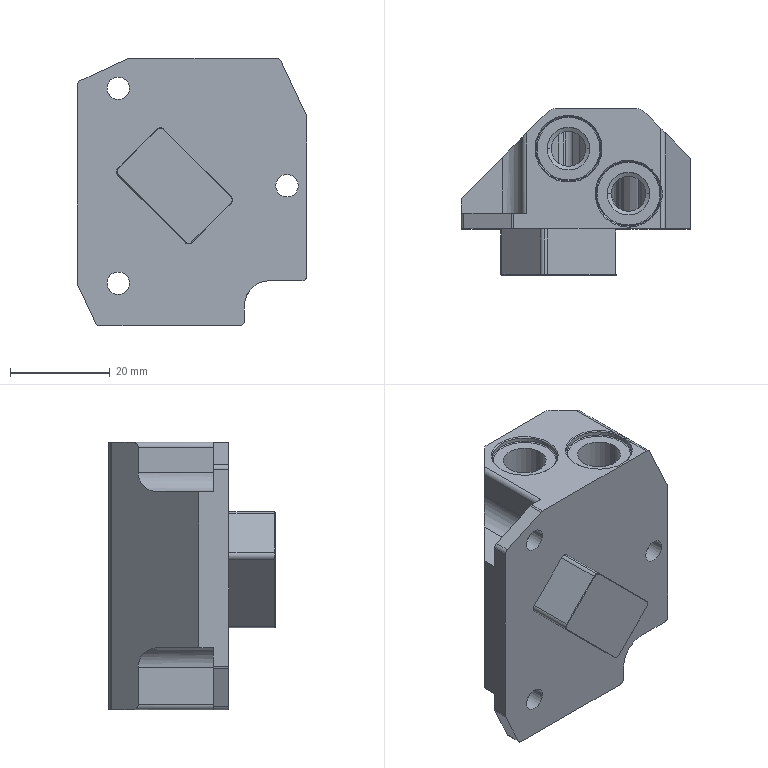NC program | NX | posted with a generic post | part box 46 x 33.25 x 53.5 mm
Lines 1 to 18 of 9227:
N10 G17 G21 G94 G90
(PLANAR_MILL , TOOL : D63面刀)
N12 T01 M6
N14 G53
N16 G17 G0 G90 X61.25 Y-5.672 B0. C0. S3500 M3
N18 G43 Z30. H1
N20 Z2.
N22 G94 G1 Z0. F800.
N24 X26.75
N26 X-26.75
N28 X-61.25
N30 Z2.
N32 G0 Z30.
N34 M5